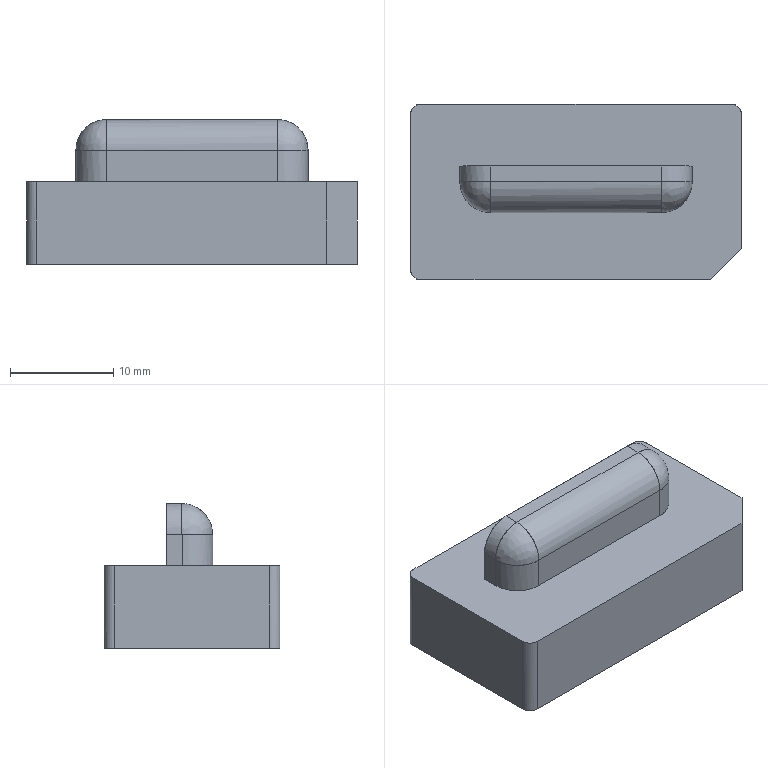NC program | PowerMill | posted with a generic post | part box 32 x 17 x 14 mm
Lines 6788 to 7532 of 64476:
N6885 M6
N6886 S22000 M03
N6887 G00 G90 X0.0 Y0.0
N6888 G43 Z10.8 H22
N6889
N6890 G05 P10000 R8
N6891 X11.5065 Y-1.9998
N6892 Z-3.6549
N6893 G01 Z-4.8549 F1200.0
N6894 X11.5064 Y-1.9999 Z-4.8359 F2000.0
N6895 X11.5061 Y-2.0002 Z-4.7481
N6896 X11.5052 Y-2.0011 Z-4.6724
N6897 X11.5043 Y-2.002 Z-4.6556
N6898 X11.5011 Y-2.0052 Z-4.637
N6899 X11.4961 Y-2.0102 Z-4.6202
N6900 X11.4874 Y-2.0189 Z-4.5995
N6901 X11.4751 Y-2.0312 Z-4.5776
N6902 X11.4577 Y-2.0486 Z-4.5522
N6903 X11.4357 Y-2.0706 Z-4.5218
N6904 X11.371 Y-2.1353 Z-4.4994
N6905 X11.3141 Y-2.1922 Z-4.513
N6906 X11.273 Y-2.2334 Z-4.5461
N6907 X11.2385 Y-2.2678 Z-4.6067
N6908 X11.2336 Y-2.2727 Z-4.6207
N6909 X11.2296 Y-2.2768 Z-4.6404
N6910 X11.2264 Y-2.2799 Z-4.6673
N6911 X11.2234 Y-2.2829 Z-4.6942
N6912 Z-4.8769
N6913 X11.1133 Y-2.3789 Z-4.8717
N6914 X11.0008 Y-2.4717 Z-4.8666
N6915 X10.8966 Y-2.5531 Z-4.862
N6916 X10.8967 Z-4.6977
N6917 X10.8987 Y-2.5511 Z-4.656
N6918 X10.9017 Y-2.548 Z-4.6144
N6919 X10.9065 Y-2.5432 Z-4.5719
N6920 X10.9133 Y-2.5364 Z-4.5313
N6921 X10.9222 Y-2.5275 Z-4.4917
N6922 X10.9329 Y-2.5169 Z-4.4528
N6923 X10.9446 Y-2.5052 Z-4.4156
N6924 X10.9582 Y-2.4915 Z-4.3799
N6925 X10.9752 Y-2.4746 Z-4.3427
N6926 X10.9959 Y-2.4539 Z-4.3043
N6927 X11.02 Y-2.4297 Z-4.2656
N6928 X11.0465 Y-2.4032 Z-4.2291
N6929 X11.0735 Y-2.3763 Z-4.1972
N6930 X11.0998 Y-2.3499 Z-4.1705
N6931 X11.1251 Y-2.3246 Z-4.1488
N6932 X11.1509 Y-2.2989 Z-4.1307
N6933 X11.184 Y-2.2657 Z-4.1113
N6934 X11.2182 Y-2.2315 Z-4.0957
N6935 X11.2532 Y-2.1965 Z-4.0839
N6936 X11.2888 Y-2.1609 Z-4.076
N6937 X11.3248 Y-2.1249 Z-4.0721
N6938 X11.3585 Y-2.0912
N6939 X11.3924 Y-2.0574 Z-4.0759
N6940 X11.4262 Y-2.0236 Z-4.0838
N6941 X11.4596 Y-1.9901 Z-4.0956
N6942 X11.4923 Y-1.9574 Z-4.1113
N6943 X11.5241 Y-1.9257 Z-4.1306
N6944 X11.5546 Y-1.8951 Z-4.1536
N6945 X11.5838 Y-1.866 Z-4.1798
N6946 X11.6111 Y-1.8387 Z-4.2088
N6947 X11.6365 Y-1.8132 Z-4.2391
N6948 X11.6603 Y-1.7894 Z-4.2716
N6949 X11.6822 Y-1.7676 Z-4.3066
N6950 X11.7013 Y-1.7484 Z-4.3431
N6951 X11.7181 Y-1.7317 Z-4.381
N6952 X11.7328 Y-1.717 Z-4.4203
N6953 X11.7453 Y-1.7045 Z-4.4594
N6954 X11.756 Y-1.6938 Z-4.5002
N6955 X11.7645 Y-1.6853 Z-4.542
N6956 X11.7708 Y-1.679 Z-4.5848
N6957 X11.7752 Y-1.6746 Z-4.6302
N6958 X11.7785 Y-1.6712 Z-4.6864
N6959 X11.7786 Y-1.6711 Z-4.6891
N6960 X11.7787 Y-1.671 Z-4.8532
N6961 X11.9152 Y-1.478 Z-4.8497
N6962 Z-4.691
N6963 X11.9149 Y-1.4783 Z-4.68
N6964 X11.9116 Y-1.4816 Z-4.6166
N6965 X11.9056 Y-1.4875 Z-4.5546
N6966 X11.8971 Y-1.4961 Z-4.4947
N6967 X11.887 Y-1.5062 Z-4.4412
N6968 X11.8739 Y-1.5193 Z-4.3876
N6969 X11.8581 Y-1.5351 Z-4.3347
N6970 X11.8402 Y-1.553 Z-4.2848
N6971 X11.8206 Y-1.5725 Z-4.2381
N6972 X11.7977 Y-1.5954 Z-4.1897
N6973 X11.7731 Y-1.6201 Z-4.1441
N6974 X11.7467 Y-1.6465 Z-4.1018
N6975 X11.7187 Y-1.6744 Z-4.0627
N6976 X11.6891 Y-1.704 Z-4.0267
N6977 X11.658 Y-1.7352 Z-3.9935
N6978 X11.6249 Y-1.7683 Z-3.9625
N6979 X11.5894 Y-1.8038 Z-3.9338
N6980 X11.5526 Y-1.8405 Z-3.9087
N6981 X11.5147 Y-1.8785 Z-3.8872
N6982 X11.4756 Y-1.9175 Z-3.8693
N6983 X11.4357 Y-1.9574 Z-3.8553
N6984 X11.3952 Y-1.998 Z-3.8451
N6985 X11.3541 Y-2.0391 Z-3.8389
N6986 X11.3128 Y-2.0804 Z-3.8366
N6987 X11.2715 Y-2.1217 Z-3.8383
N6988 X11.2304 Y-2.1628 Z-3.844
N6989 X11.19 Y-2.2032 Z-3.8536
N6990 X11.1501 Y-2.2431 Z-3.867
N6991 X11.1109 Y-2.2823 Z-3.8844
N6992 X11.0726 Y-2.3206 Z-3.9055
N6993 X11.0353 Y-2.3579 Z-3.9303
N6994 X10.9992 Y-2.3939 Z-3.9587
N6995 X10.9646 Y-2.4285 Z-3.9906
N6996 X10.9317 Y-2.4615 Z-4.0256
N6997 X10.9004 Y-2.4927 Z-4.0639
N6998 X10.8711 Y-2.5221 Z-4.1051
N6999 X10.8437 Y-2.5494 Z-4.149
N7000 X10.8185 Y-2.5747 Z-4.1957
N7001 X10.7955 Y-2.5977 Z-4.2447
N7002 X10.7749 Y-2.6183 Z-4.296
N7003 X10.7567 Y-2.6364 Z-4.3491
N7004 X10.7412 Y-2.652 Z-4.4038
N7005 X10.7283 Y-2.6649 Z-4.4599
N7006 X10.718 Y-2.6751 Z-4.5171
N7007 X10.7105 Y-2.6827 Z-4.5751
N7008 X10.7057 Y-2.6874 Z-4.6338
N7009 X10.7037 Y-2.6894 Z-4.6929
N7010 Y-2.6895 Z-4.8562
N7011 X10.5482 Y-2.7884 Z-4.8553
N7012 Z-4.6812
N7013 X10.5506 Y-2.786 Z-4.6155
N7014 X10.5558 Y-2.7808 Z-4.5504
N7015 X10.5638 Y-2.7728 Z-4.4862
N7016 X10.5745 Y-2.7621 Z-4.4231
N7017 X10.5879 Y-2.7487 Z-4.3612
N7018 X10.6038 Y-2.7328 Z-4.3009
N7019 X10.6224 Y-2.7142 Z-4.2422
N7020 X10.6434 Y-2.6932 Z-4.1854
N7021 X10.6668 Y-2.6698 Z-4.1307
N7022 X10.6925 Y-2.6441 Z-4.0781
N7023 X10.7205 Y-2.6161 Z-4.0278
N7024 X10.7508 Y-2.5858 Z-3.9797
N7025 X10.7828 Y-2.5538 Z-3.9346
N7026 X10.8165 Y-2.5201 Z-3.8924
N7027 X10.852 Y-2.4846 Z-3.8533
N7028 X10.889 Y-2.4476 Z-3.8174
N7029 X10.9275 Y-2.4091 Z-3.7849
N7030 X10.9674 Y-2.3692 Z-3.7557
N7031 X11.0087 Y-2.3279 Z-3.73
N7032 X11.0511 Y-2.2855 Z-3.7079
N7033 X11.0946 Y-2.242 Z-3.6895
N7034 X11.1391 Y-2.1975 Z-3.6748
N7035 X11.1843 Y-2.1523 Z-3.664
N7036 X11.2286 Y-2.1079 Z-3.6573
N7037 X11.2732 Y-2.0634 Z-3.6545
N7038 X11.3178 Y-2.0188 Z-3.6556
N7039 X11.3624 Y-1.9742 Z-3.6607
N7040 X11.4069 Y-1.9297 Z-3.6697
N7041 X11.4509 Y-1.8857 Z-3.6826
N7042 X11.4945 Y-1.8421 Z-3.6994
N7043 X11.5374 Y-1.7992 Z-3.7201
N7044 X11.5795 Y-1.7571 Z-3.7445
N7045 X11.6204 Y-1.7162 Z-3.7727
N7046 X11.6601 Y-1.6765 Z-3.8043
N7047 X11.6983 Y-1.6383 Z-3.8394
N7048 X11.7348 Y-1.6018 Z-3.8777
N7049 X11.7694 Y-1.5672 Z-3.9189
N7050 X11.8002 Y-1.5364 Z-3.9605
N7051 X11.8303 Y-1.5063 Z-4.0064
N7052 X11.8593 Y-1.4773 Z-4.0564
N7053 X11.8861 Y-1.4505 Z-4.1086
N7054 X11.9097 Y-1.4269 Z-4.1613
N7055 X11.9302 Y-1.4064 Z-4.214
N7056 X11.9486 Y-1.388 Z-4.2682
N7057 X11.9657 Y-1.3709 Z-4.3263
N7058 X11.9804 Y-1.3562 Z-4.3856
N7059 X11.9925 Y-1.3441 Z-4.446
N7060 X12.0018 Y-1.3348 Z-4.5075
N7061 X12.0085 Y-1.3281 Z-4.5697
N7062 X12.0126 Y-1.324 Z-4.6326
N7063 X12.0144 Y-1.3222 Z-4.6904
N7064 X12.0145 Y-1.3221 Z-4.8542
N7065 X12.0937 Y-1.1864 Z-4.8586
N7066 X12.0936 Z-4.6881
N7067 X12.0926 Y-1.1874 Z-4.642
N7068 X12.0895 Y-1.1906 Z-4.5798
N7069 X12.084 Y-1.196 Z-4.5179
N7070 X12.0757 Y-1.2043 Z-4.4546
N7071 X12.0653 Y-1.2147 Z-4.394
N7072 X12.0529 Y-1.2271 Z-4.3341
N7073 X12.0387 Y-1.2413 Z-4.275
N7074 X12.0206 Y-1.2594 Z-4.2111
N7075 X12.0001 Y-1.28 Z-4.1492
N7076 X11.9771 Y-1.3029 Z-4.0894
N7077 X11.9517 Y-1.3283 Z-4.0316
N7078 X11.9238 Y-1.3562 Z-3.9756
N7079 X11.8934 Y-1.3866 Z-3.9216
N7080 X11.8622 Y-1.4179 Z-3.872
N7081 X11.8289 Y-1.4511 Z-3.8248
N7082 X11.7932 Y-1.4869 Z-3.7798
N7083 X11.755 Y-1.5251 Z-3.737
N7084 X11.7153 Y-1.5647 Z-3.6975
N7085 X11.6743 Y-1.6058 Z-3.6614
N7086 X11.6318 Y-1.6482 Z-3.6287
N7087 X11.5881 Y-1.6919 Z-3.5995
N7088 X11.5432 Y-1.7368 Z-3.574
N7089 X11.4973 Y-1.7827 Z-3.5521
N7090 X11.4506 Y-1.8294 Z-3.5341
N7091 X11.4032 Y-1.8769 Z-3.5199
N7092 X11.3552 Y-1.9248 Z-3.5097
N7093 X11.3069 Y-1.9731 Z-3.5034
N7094 X11.2584 Y-2.0216 Z-3.5011
N7095 X11.2099 Y-2.0701 Z-3.5028
N7096 X11.1616 Y-2.1184 Z-3.5085
N7097 X11.1137 Y-2.1664 Z-3.5181
N7098 X11.0662 Y-2.2138 Z-3.5316
N7099 X11.0193 Y-2.2607 Z-3.549
N7100 X10.9733 Y-2.3067 Z-3.5701
N7101 X10.9281 Y-2.3519 Z-3.5951
N7102 X10.884 Y-2.3961 Z-3.6238
N7103 X10.8409 Y-2.4391 Z-3.6561
N7104 X10.7992 Y-2.4808 Z-3.692
N7105 X10.7589 Y-2.5212 Z-3.7314
N7106 X10.7201 Y-2.5599 Z-3.774
N7107 X10.6836 Y-2.5964 Z-3.8192
N7108 X10.6489 Y-2.6312 Z-3.8674
N7109 X10.6162 Y-2.6638 Z-3.9183
N7110 X10.5857 Y-2.6944 Z-3.9718
N7111 X10.5574 Y-2.7227 Z-4.0277
N7112 X10.5313 Y-2.7487 Z-4.086
N7113 X10.5076 Y-2.7724 Z-4.1464
N7114 X10.4864 Y-2.7936 Z-4.2088
N7115 X10.4677 Y-2.8123 Z-4.2729
N7116 X10.4517 Y-2.8284 Z-4.3385
N7117 X10.4383 Y-2.8417 Z-4.4054
N7118 X10.4276 Y-2.8524 Z-4.4732
N7119 X10.4198 Y-2.8603 Z-4.5418
N7120 X10.4147 Y-2.8653 Z-4.6109
N7121 X10.4124 Y-2.8676 Z-4.6803
N7122 Y-2.8677 Z-4.851
N7123 X10.2897 Y-2.9337 Z-4.8504
N7124 X10.2898 Z-4.6803
N7125 X10.2921 Y-2.9313 Z-4.6058
N7126 X10.2973 Y-2.9262 Z-4.5321
N7127 X10.3051 Y-2.9183 Z-4.4594
N7128 X10.3157 Y-2.9078 Z-4.3879
N7129 X10.3289 Y-2.8946 Z-4.3179
N7130 X10.3447 Y-2.8787 Z-4.2494
N7131 X10.3631 Y-2.8604 Z-4.1827
N7132 X10.384 Y-2.8395 Z-4.1176
N7133 X10.4081 Y-2.8154 Z-4.0521
N7134 X10.4346 Y-2.7889 Z-3.9886
N7135 X10.4634 Y-2.7601 Z-3.9275
N7136 X10.4944 Y-2.729 Z-3.8688
N7137 X10.5276 Y-2.6959 Z-3.8128
N7138 X10.5628 Y-2.6607 Z-3.7596
N7139 X10.5998 Y-2.6237 Z-3.7093
N7140 X10.6387 Y-2.5847 Z-3.6621
N7141 X10.6794 Y-2.544 Z-3.6179
N7142 X10.7218 Y-2.5016 Z-3.5769
N7143 X10.7657 Y-2.4577 Z-3.5393
N7144 X10.8111 Y-2.4124 Z-3.5052
N7145 X10.8578 Y-2.3657 Z-3.4745
N7146 X10.9056 Y-2.3179 Z-3.4475
N7147 X10.9544 Y-2.269 Z-3.4243
N7148 X11.0041 Y-2.2194 Z-3.4048
N7149 X11.0544 Y-2.1691 Z-3.3893
N7150 X11.1052 Y-2.1183 Z-3.3776
N7151 X11.1538 Y-2.0696 Z-3.3702
N7152 X11.2029 Y-2.0205 Z-3.3666
N7153 X11.2532 Y-1.9703 Z-3.3669
N7154 X11.3046 Y-1.9188 Z-3.3711
N7155 X11.3551 Y-1.8684 Z-3.379
N7156 X11.4052 Y-1.8182 Z-3.3908
N7157 X11.4549 Y-1.7686 Z-3.4065
N7158 X11.5038 Y-1.7196 Z-3.4261
N7159 X11.552 Y-1.6714 Z-3.4495
N7160 X11.5993 Y-1.6241 Z-3.4767
N7161 X11.6456 Y-1.5779 Z-3.5076
N7162 X11.6906 Y-1.5328 Z-3.5422
N7163 X11.7343 Y-1.4892 Z-3.5802
N7164 X11.7764 Y-1.4471 Z-3.6215
N7165 X11.8169 Y-1.4066 Z-3.6661
N7166 X11.8555 Y-1.3679 Z-3.7137
N7167 X11.8923 Y-1.3311 Z-3.7644
N7168 X11.9272 Y-1.2963 Z-3.8178
N7169 X11.9598 Y-1.2637 Z-3.8738
N7170 X11.9901 Y-1.2333 Z-3.9321
N7171 X12.0181 Y-1.2053 Z-3.9927
N7172 X12.044 Y-1.1795 Z-4.0558
N7173 X12.0674 Y-1.156 Z-4.1211
N7174 X12.0885 Y-1.135 Z-4.1884
N7175 X12.107 Y-1.1165 Z-4.2575
N7176 X12.1229 Y-1.1006 Z-4.3283
N7177 X12.1351 Y-1.0884 Z-4.3945
N7178 X12.1448 Y-1.0786 Z-4.4629
N7179 X12.1522 Y-1.0712 Z-4.5345
N7180 X12.1572 Y-1.0663 Z-4.6096
N7181 X12.1593 Y-1.0642 Z-4.6712
N7182 Y-1.0641 Z-4.8602
N7183 X12.2164 Y-0.9505 Z-4.8613
N7184 Z-4.6895
N7185 X12.2155 Y-0.9514 Z-4.6452
N7186 X12.2118 Y-0.9551 Z-4.5669
N7187 X12.2053 Y-0.9616 Z-4.4894
N7188 X12.1961 Y-0.9708 Z-4.413
N7189 X12.1842 Y-0.9827 Z-4.3378
N7190 X12.1697 Y-0.9972 Z-4.264
N7191 X12.1525 Y-1.0144 Z-4.1918
N7192 X12.1328 Y-1.0341 Z-4.1213
N7193 X12.1106 Y-1.0563 Z-4.0525
N7194 X12.0858 Y-1.0811 Z-3.9853
N7195 X12.0585 Y-1.1084 Z-3.92
N7196 X12.0288 Y-1.1381 Z-3.8567
N7197 X11.9966 Y-1.1703 Z-3.7956
N7198 X11.9622 Y-1.2047 Z-3.7367
N7199 X11.9255 Y-1.2414 Z-3.6801
N7200 X11.8877 Y-1.2791 Z-3.6278
N7201 X11.8481 Y-1.3188 Z-3.5783
N7202 X11.8066 Y-1.3603 Z-3.5318
N7203 X11.7632 Y-1.4037 Z-3.4883
N7204 X11.7181 Y-1.4488 Z-3.4479
N7205 X11.6715 Y-1.4954 Z-3.4109
N7206 X11.6234 Y-1.5434 Z-3.3774
N7207 X11.5741 Y-1.5928 Z-3.3474
N7208 X11.5238 Y-1.6431 Z-3.3211
N7209 X11.4726 Y-1.6943 Z-3.2986
N7210 X11.4207 Y-1.7462 Z-3.2801
N7211 X11.3682 Y-1.7987 Z-3.2654
N7212 X11.3155 Y-1.8514 Z-3.2547
N7213 X11.2625 Y-1.9044 Z-3.2479
N7214 X11.2096 Y-1.9573 Z-3.2451
N7215 X11.1567 Y-2.0102 Z-3.2463
N7216 X11.1041 Y-2.0628 Z-3.2515
N7217 X11.0504 Y-2.1165 Z-3.2606
N7218 X10.9974 Y-2.1695 Z-3.2737
N7219 X10.9453 Y-2.2216 Z-3.2906
N7220 X10.8941 Y-2.2728 Z-3.3113
N7221 X10.8438 Y-2.3231 Z-3.3357
N7222 X10.7944 Y-2.3725 Z-3.3639
N7223 X10.7461 Y-2.4208 Z-3.3959
N7224 X10.6988 Y-2.4681 Z-3.4315
N7225 X10.6545 Y-2.5124 Z-3.4692
N7226 X10.6102 Y-2.5567 Z-3.5114
N7227 X10.5665 Y-2.6004 Z-3.5577
N7228 X10.5248 Y-2.6421 Z-3.6069
N7229 X10.486 Y-2.6809 Z-3.6576
N7230 X10.4502 Y-2.7167 Z-3.7096
N7231 X10.4166 Y-2.7503 Z-3.7638
N7232 X10.3834 Y-2.7835 Z-3.8233
N7233 X10.352 Y-2.8149 Z-3.8859
N7234 X10.3228 Y-2.8441 Z-3.9511
N7235 X10.296 Y-2.8709 Z-4.0184
N7236 X10.2718 Y-2.895 Z-4.0871
N7237 X10.2505 Y-2.9164 Z-4.1567
N7238 X10.232 Y-2.9349 Z-4.2268
N7239 X10.2165 Y-2.9504 Z-4.2967
N7240 X10.205 Y-2.9619 Z-4.3595
N7241 X10.1953 Y-2.9716 Z-4.4229
N7242 X10.1874 Y-2.9794 Z-4.4868
N7243 X10.1819 Y-2.985 Z-4.5512
N7244 X10.1784 Y-2.9885 Z-4.6159
N7245 X10.1765 Y-2.9904 Z-4.6807
N7246 X10.1764 Z-4.8487
N7247 X10.0707 Y-3.0396 Z-4.8465
N7248 Z-4.6866
N7249 X10.0723 Y-3.0381 Z-4.6113
N7250 X10.0766 Y-3.0337 Z-4.5349
N7251 X10.0838 Y-3.0265 Z-4.4575
N7252 X10.0939 Y-3.0164 Z-4.3798
N7253 X10.1068 Y-3.0035 Z-4.3022
N7254 X10.1226 Y-2.9878 Z-4.2253
N7255 X10.1409 Y-2.9694 Z-4.1499
N7256 X10.1617 Y-2.9486 Z-4.0764
N7257 X10.1849 Y-2.9255 Z-4.0053
N7258 X10.2101 Y-2.9002 Z-3.9371
N7259 X10.2376 Y-2.8727 Z-3.8712
N7260 X10.2685 Y-2.8418 Z-3.8047
N7261 X10.3018 Y-2.8086 Z-3.7405
N7262 X10.3372 Y-2.7731 Z-3.6789
N7263 X10.3747 Y-2.7357 Z-3.62
N7264 X10.4141 Y-2.6962 Z-3.564
N7265 X10.4554 Y-2.6549 Z-3.511
N7266 X10.4984 Y-2.6119 Z-3.4611
N7267 X10.5431 Y-2.5672 Z-3.4145
N7268 X10.5892 Y-2.5211 Z-3.3713
N7269 X10.6369 Y-2.4735 Z-3.3314
N7270 X10.6858 Y-2.4245 Z-3.2951
N7271 X10.7366 Y-2.3737 Z-3.2618
N7272 X10.7884 Y-2.3219 Z-3.2323
N7273 X10.841 Y-2.2693 Z-3.2066
N7274 X10.8943 Y-2.216 Z-3.1848
N7275 X10.948 Y-2.1623 Z-3.1669
N7276 X11.0021 Y-2.1082 Z-3.153
N7277 X11.0564 Y-2.054 Z-3.1431
N7278 X11.1108 Y-1.9995 Z-3.1371
N7279 X11.1671 Y-1.9432 Z-3.1348
N7280 X11.223 Y-1.8873 Z-3.1364
N7281 X11.2783 Y-1.8321 Z-3.1419
N7282 X11.333 Y-1.7773 Z-3.1514
N7283 X11.3871 Y-1.7232 Z-3.1648
N7284 X11.4405 Y-1.6698 Z-3.1821
N7285 X11.4933 Y-1.6171 Z-3.2032
N7286 X11.5453 Y-1.5651 Z-3.2282
N7287 X11.5965 Y-1.5138 Z-3.257
N7288 X11.6469 Y-1.4634 Z-3.2896
N7289 X11.6965 Y-1.4138 Z-3.326
N7290 X11.7441 Y-1.3662 Z-3.3652
N7291 X11.7899 Y-1.3204 Z-3.4073
N7292 X11.8339 Y-1.2764 Z-3.4523
N7293 X11.8761 Y-1.2342 Z-3.5004
N7294 X11.9166 Y-1.1937 Z-3.5515
N7295 X11.9554 Y-1.1549 Z-3.6059
N7296 X11.9926 Y-1.1178 Z-3.6636
N7297 X12.0281 Y-1.0822 Z-3.7246
N7298 X12.0622 Y-1.0482 Z-3.7891
N7299 X12.0918 Y-1.0185 Z-3.8512
N7300 X12.1195 Y-0.9908 Z-3.9163
N7301 X12.1454 Y-0.9649 Z-3.9849
N7302 X12.1694 Y-0.9409 Z-4.0567
N7303 X12.1914 Y-0.9189 Z-4.1319
N7304 X12.208 Y-0.9023 Z-4.1966
N7305 X12.2223 Y-0.888 Z-4.2623
N7306 X12.2353 Y-0.875 Z-4.3338
N7307 X12.2469 Y-0.8635 Z-4.412
N7308 X12.2558 Y-0.8545 Z-4.4912
N7309 X12.2617 Y-0.8487 Z-4.5651
N7310 X12.2648 Y-0.8455 Z-4.6337
N7311 X12.2655 Y-0.8448 Z-4.6832
N7312 Z-4.8593
N7313 X12.3092 Y-0.7445 Z-4.8621
N7314 Y-0.7446 Z-4.6874
N7315 X12.3079 Y-0.7459 Z-4.6179
N7316 X12.3038 Y-0.7499 Z-4.5385
N7317 X12.2969 Y-0.7569 Z-4.4577
N7318 X12.287 Y-0.7667 Z-4.3762
N7319 X12.2743 Y-0.7794 Z-4.2947
N7320 X12.259 Y-0.7948 Z-4.2146
N7321 X12.2412 Y-0.8126 Z-4.1369
N7322 X12.2212 Y-0.8325 Z-4.0621
N7323 X12.1997 Y-0.8541 Z-3.9918
N7324 X12.1754 Y-0.8784 Z-3.9219
N7325 X12.1477 Y-0.9061 Z-3.8509
N7326 X12.1169 Y-0.9369 Z-3.7802
N7327 X12.0841 Y-0.9696 Z-3.7124
N7328 X12.0502 Y-1.0035 Z-3.649
N7329 X12.0158 Y-1.038 Z-3.5907
N7330 X11.9798 Y-1.074 Z-3.5357
N7331 X11.9387 Y-1.115 Z-3.4784
N7332 X11.8962 Y-1.1576 Z-3.4244
N7333 X11.8522 Y-1.2016 Z-3.374
N7334 X11.8067 Y-1.247 Z-3.3269
N7335 X11.7598 Y-1.294 Z-3.2832
N7336 X11.7112 Y-1.3425 Z-3.2425
N7337 X11.6604 Y-1.3934 Z-3.2043
N7338 X11.6086 Y-1.4451 Z-3.1699
N7339 X11.556 Y-1.4977 Z-3.1393
N7340 X11.5026 Y-1.5512 Z-3.1126
N7341 X11.4483 Y-1.6055 Z-3.0896
N7342 X11.3932 Y-1.6606 Z-3.0705
N7343 X11.3373 Y-1.7164 Z-3.0552
N7344 X11.2807 Y-1.7731 Z-3.0437
N7345 X11.2233 Y-1.8305 Z-3.0362
N7346 X11.1652 Y-1.8886 Z-3.0325
N7347 X11.1063 Y-1.9474 Z-3.0327
N7348 X11.0568 Y-1.9969 Z-3.0361
N7349 X11.0075 Y-2.0463 Z-3.043
N7350 X10.9536 Y-2.1001 Z-3.054
N7351 X10.8963 Y-2.1575 Z-3.0696
N7352 X10.8445 Y-2.2092 Z-3.0871
N7353 X10.7969 Y-2.2569 Z-3.1064
N7354 X10.7499 Y-2.3039 Z-3.1288
N7355 X10.6955 Y-2.3583 Z-3.1588
N7356 X10.6424 Y-2.4114 Z-3.1923
N7357 X10.5907 Y-2.463 Z-3.2293
N7358 X10.5406 Y-2.5131 Z-3.2696
N7359 X10.4922 Y-2.5616 Z-3.3132
N7360 X10.4454 Y-2.6083 Z-3.3599
N7361 X10.4008 Y-2.6529 Z-3.4093
N7362 X10.3576 Y-2.6961 Z-3.4622
N7363 X10.3158 Y-2.7379 Z-3.5187
N7364 X10.2755 Y-2.7783 Z-3.5787
N7365 X10.239 Y-2.8148 Z-3.6384
N7366 X10.2043 Y-2.8494 Z-3.701
N7367 X10.1714 Y-2.8824 Z-3.767
N7368 X10.1403 Y-2.9135 Z-3.8363
N7369 X10.1116 Y-2.9422 Z-3.9074
N7370 X10.0855 Y-2.9683 Z-3.9802
N7371 X10.0619 Y-2.9918 Z-4.0545
N7372 X10.041 Y-3.0127 Z-4.1303
N7373 X10.0228 Y-3.031 Z-4.2074
N7374 X10.0072 Y-3.0465 Z-4.2858
N7375 X9.9944 Y-3.0594 Z-4.3654
N7376 X9.9842 Y-3.0695 Z-4.4461
N7377 X9.9768 Y-3.077 Z-4.5278
N7378 X9.9722 Y-3.0816 Z-4.6104
N7379 X9.9703 Y-3.0835 Z-4.6937
N7380 X9.9702 Z-4.8448
N7381 X9.8749 Y-3.1223 Z-4.8454
N7382 X9.875 Y-3.1222 Z-4.6989
N7383 X9.8766 Y-3.1206 Z-4.6133
N7384 X9.881 Y-3.1162 Z-4.5287
N7385 X9.8882 Y-3.109 Z-4.4453
N7386 X9.898 Y-3.0992 Z-4.3633
N7387 X9.9105 Y-3.0867 Z-4.2827
N7388 X9.9256 Y-3.0716 Z-4.2035
N7389 X9.9437 Y-3.0535 Z-4.1227
N7390 X9.964 Y-3.0332 Z-4.0446
N7391 X9.9866 Y-3.0105 Z-3.969
N7392 X10.0116 Y-2.9856 Z-3.8959
N7393 X10.0388 Y-2.9584 Z-3.825
N7394 X10.0682 Y-2.929 Z-3.7562
N7395 X10.0982 Y-2.899 Z-3.6923
N7396 X10.1298 Y-2.8674 Z-3.6301
N7397 X10.1634 Y-2.8338 Z-3.57
N7398 X10.199 Y-2.7982 Z-3.5121
N7399 X10.2364 Y-2.7608 Z-3.4566
N7400 X10.2753 Y-2.7219 Z-3.4033
N7401 X10.3178 Y-2.6794 Z-3.3498
N7402 X10.3629 Y-2.6343 Z-3.2984
N7403 X10.4102 Y-2.587 Z-3.2496
N7404 X10.4597 Y-2.5375 Z-3.2036
N7405 X10.5109 Y-2.4863 Z-3.1606
N7406 X10.5635 Y-2.4337 Z-3.1211
N7407 X10.6172 Y-2.38 Z-3.0854
N7408 X10.6715 Y-2.3257 Z-3.0535
N7409 X10.7263 Y-2.2709 Z-3.0257
N7410 X10.7828 Y-2.2144 Z-3.0011
N7411 X10.84 Y-2.1572 Z-2.9805
N7412 X10.8976 Y-2.0996 Z-2.9638
N7413 X10.9556 Y-2.0416 Z-2.9511
N7414 X11.0138 Y-1.9834 Z-2.9423
N7415 X11.0721 Y-1.9251 Z-2.9376
N7416 X11.1304 Y-1.8668 Z-2.9368
N7417 X11.1896 Y-1.8076 Z-2.9398
N7418 X11.2484 Y-1.7488 Z-2.9469
N7419 X11.3069 Y-1.6903 Z-2.9578
N7420 X11.3648 Y-1.6324 Z-2.9727
N7421 X11.4221 Y-1.5751 Z-2.9915
N7422 X11.4786 Y-1.5186 Z-3.0141
N7423 X11.5343 Y-1.4629 Z-3.0405
N7424 X11.5889 Y-1.4082 Z-3.0707
N7425 X11.6425 Y-1.3547 Z-3.1045
N7426 X11.6949 Y-1.3023 Z-3.142
N7427 X11.7459 Y-1.2513 Z-3.1829
N7428 X11.7956 Y-1.2016 Z-3.2274
N7429 X11.8437 Y-1.1535 Z-3.2752
N7430 X11.8903 Y-1.1069 Z-3.3262
N7431 X11.9341 Y-1.0631 Z-3.3791
N7432 X11.9771 Y-1.0201 Z-3.4361
N7433 X12.0179 Y-0.9793 Z-3.4958
N7434 X12.0565 Y-0.9407 Z-3.5578
N7435 X12.0927 Y-0.9045 Z-3.6219
N7436 X12.1262 Y-0.8709 Z-3.6878
N7437 X12.1568 Y-0.8403 Z-3.7544
N7438 X12.1819 Y-0.8153 Z-3.8133
N7439 X12.2056 Y-0.7916 Z-3.8733
N7440 X12.2274 Y-0.7698 Z-3.9347
N7441 X12.2471 Y-0.7501 Z-3.9975
N7442 X12.2651 Y-0.732 Z-4.0613
N7443 X12.2816 Y-0.7155 Z-4.1259
N7444 X12.2981 Y-0.6991 Z-4.2012
N7445 X12.3129 Y-0.6843 Z-4.2822
N7446 X12.3257 Y-0.6715 Z-4.3667
N7447 X12.3355 Y-0.6617 Z-4.4501
N7448 X12.3425 Y-0.6547 Z-4.5323
N7449 X12.3465 Y-0.6507 Z-4.6133
N7450 X12.3477 Y-0.6495 Z-4.6697
N7451 Z-4.8706
N7452 X12.3822 Y-0.5584 Z-4.8755
N7453 X12.3821 Y-0.5585 Z-4.6534
N7454 X12.3811 Y-0.5595 Z-4.6137
N7455 X12.3774 Y-0.5633 Z-4.533
N7456 X12.3712 Y-0.5695 Z-4.4525
N7457 X12.3624 Y-0.5782 Z-4.3725
N7458 X12.3512 Y-0.5894 Z-4.2932
N7459 X12.3377 Y-0.6029 Z-4.2145
N7460 X12.3208 Y-0.6198 Z-4.1318
N7461 X12.3012 Y-0.6394 Z-4.0502
N7462 X12.2789 Y-0.6617 Z-3.97
N7463 X12.254 Y-0.6866 Z-3.8914
N7464 X12.2266 Y-0.714 Z-3.8146
N7465 X12.1968 Y-0.7439 Z-3.7398
N7466 X12.1644 Y-0.7762 Z-3.6669
N7467 X12.1298 Y-0.8108 Z-3.5963
N7468 X12.0931 Y-0.8475 Z-3.5285
N7469 X12.0542 Y-0.8864 Z-3.4632
N7470 X12.0132 Y-0.9274 Z-3.4006
N7471 X11.9702 Y-0.9704 Z-3.3407
N7472 X11.9252 Y-1.0154 Z-3.2838
N7473 X11.8784 Y-1.0622 Z-3.2299
N7474 X11.8299 Y-1.1108 Z-3.1791
N7475 X11.7797 Y-1.161 Z-3.1316
N7476 X11.7279 Y-1.2127 Z-3.0875
N7477 X11.6748 Y-1.2658 Z-3.0468
N7478 X11.6205 Y-1.3202 Z-3.0097
N7479 X11.5649 Y-1.3757 Z-2.9762
N7480 X11.5084 Y-1.4323 Z-2.9465
N7481 X11.4509 Y-1.4897 Z-2.9205
N7482 X11.3926 Y-1.548 Z-2.8984
N7483 X11.3343 Y-1.6063 Z-2.8803
N7484 X11.2754 Y-1.6652 Z-2.8661
N7485 X11.2157 Y-1.7249 Z-2.8557
N7486 X11.1553 Y-1.7853 Z-2.8493
N7487 X11.0944 Y-1.8462 Z-2.8468
N7488 X11.0346 Y-1.906 Z-2.8482
N7489 X10.9748 Y-1.9658 Z-2.8537
N7490 X10.9149 Y-2.0257 Z-2.8631
N7491 X10.8551 Y-2.0855 Z-2.8765
N7492 X10.7956 Y-2.145 Z-2.8939
N7493 X10.7365 Y-2.2042 Z-2.9153
N7494 X10.6791 Y-2.2615 Z-2.9401
N7495 X10.6224 Y-2.3182 Z-2.9688
N7496 X10.5665 Y-2.3741 Z-3.0013
N7497 X10.5116 Y-2.429 Z-3.0375
N7498 X10.4578 Y-2.4828 Z-3.0774
N7499 X10.4054 Y-2.5352 Z-3.1209
N7500 X10.3545 Y-2.5861 Z-3.1676
N7501 X10.3054 Y-2.6352 Z-3.2175
N7502 X10.2581 Y-2.6825 Z-3.2705
N7503 X10.2122 Y-2.7284 Z-3.3269
N7504 X10.1682 Y-2.7724 Z-3.3863
N7505 X10.1262 Y-2.8144 Z-3.4485
N7506 X10.0863 Y-2.8544 Z-3.5134
N7507 X10.0485 Y-2.8921 Z-3.5809
N7508 X10.0131 Y-2.9275 Z-3.6507
N7509 X9.98 Y-2.9606 Z-3.7226
N7510 X9.9494 Y-2.9913 Z-3.7966
N7511 X9.9212 Y-3.0194 Z-3.8725
N7512 X9.8956 Y-3.045 Z-3.9501
N7513 X9.8732 Y-3.0674 Z-4.0269
N7514 X9.8533 Y-3.0873 Z-4.1041
N7515 X9.8357 Y-3.1049 Z-4.1826
N7516 X9.8205 Y-3.1201 Z-4.2625
N7517 X9.8079 Y-3.1327 Z-4.3439
N7518 X9.798 Y-3.1426 Z-4.4268
N7519 X9.7908 Y-3.1498 Z-4.5105
N7520 X9.7862 Y-3.1544 Z-4.5948
N7521 X9.784 Y-3.1567 Z-4.6795
N7522 X9.7839 Z-4.8459
N7523 X9.6961 Y-3.1879 Z-4.8559
N7524 X9.6962 Y-3.1878 Z-4.6808
N7525 X9.6984 Y-3.1856 Z-4.5913
N7526 X9.7034 Y-3.1806 Z-4.5027
N7527 X9.7111 Y-3.1729 Z-4.4151
N7528 X9.7216 Y-3.1625 Z-4.3285
N7529 X9.7347 Y-3.1493 Z-4.2428
N7530 X9.7507 Y-3.1333 Z-4.1579
N7531 X9.7694 Y-3.1146 Z-4.0738
N7532 X9.7909 Y-3.0931 Z-3.9906
N7533 X9.8152 Y-3.0688 Z-3.9081
N7534 X9.8401 Y-3.044 Z-3.8332
N7535 X9.8679 Y-3.0162 Z-3.7586
N7536 X9.8989 Y-2.9851 Z-3.6837
N7537 X9.933 Y-2.951 Z-3.6093
N7538 X9.9698 Y-2.9142 Z-3.5362
N7539 X10.0087 Y-2.8754 Z-3.4659
N7540 X10.0489 Y-2.8351 Z-3.3994
N7541 X10.0901 Y-2.794 Z-3.3372
N7542 X10.1319 Y-2.7521 Z-3.2794
N7543 X10.1756 Y-2.7084 Z-3.2244
N7544 X10.2229 Y-2.6612 Z-3.17
N7545 X10.2729 Y-2.6112 Z-3.1176
N7546 X10.3251 Y-2.5589 Z-3.0678
N7547 X10.379 Y-2.5051 Z-3.0212
N7548 X10.4337 Y-2.4504 Z-2.9786
N7549 X10.4887 Y-2.3954 Z-2.9401
N7550 X10.5435 Y-2.3406 Z-2.9061
N7551 X10.599 Y-2.285 Z-2.8758
N7552 X10.6577 Y-2.2264 Z-2.8479
N7553 X10.717 Y-2.1671 Z-2.824
N7554 X10.7769 Y-2.1072 Z-2.8039
N7555 X10.8374 Y-2.0466 Z-2.7878
N7556 X10.8986 Y-1.9854 Z-2.7755
N7557 X10.9604 Y-1.9236 Z-2.7671
N7558 X11.0223 Y-1.8618 Z-2.7627
N7559 X11.0841 Y-1.7999 Z-2.7622
N7560 X11.1457 Y-1.7383 Z-2.7657
N7561 X11.207 Y-1.677 Z-2.7732
N7562 X11.2679 Y-1.6162 Z-2.7846
N7563 X11.3283 Y-1.5558 Z-2.8
N7564 X11.3881 Y-1.4959 Z-2.8193
N7565 X11.4473 Y-1.4367 Z-2.8424
N7566 X11.5058 Y-1.3783 Z-2.8693
N7567 X11.5639 Y-1.3201 Z-2.9002
N7568 X11.6207 Y-1.2633 Z-2.9346
N7569 X11.6761 Y-1.2079 Z-2.9725
N7570 X11.7301 Y-1.154 Z-3.0139
N7571 X11.7826 Y-1.1014 Z-3.0587
N7572 X11.8337 Y-1.0504 Z-3.1069
N7573 X11.8832 Y-1.0009 Z-3.1584
N7574 X11.9312 Y-0.9529 Z-3.2133
N7575 X11.9776 Y-0.9065 Z-3.2715
N7576 X12.0211 Y-0.863 Z-3.3313
N7577 X12.0628 Y-0.8212 Z-3.3942
N7578 X12.1028 Y-0.7812 Z-3.4603
N7579 X12.141 Y-0.7431 Z-3.5294
N7580 X12.1772 Y-0.7069 Z-3.6015
N7581 X12.2113 Y-0.6727 Z-3.6764
N7582 X12.2416 Y-0.6424 Z-3.7498
N7583 X12.2697 Y-0.6143 Z-3.8259
N7584 X12.2957 Y-0.5883 Z-3.9048
N7585 X12.3196 Y-0.5645 Z-3.9865
N7586 X12.3409 Y-0.5432 Z-4.07
N7587 X12.3596 Y-0.5245 Z-4.1548
N7588 X12.3755 Y-0.5085 Z-4.2408
N7589 X12.3887 Y-0.4953 Z-4.3277
N7590 X12.3992 Y-0.4849 Z-4.4153
N7591 X12.4068 Y-0.4772 Z-4.5035
N7592 X12.4116 Y-0.4724 Z-4.592
N7593 X12.4136 Y-0.4704 Z-4.6806
N7594 Z-4.6815
N7595 X12.4137 Z-4.8778
N7596 X12.4417 Y-0.3858 Z-4.8798
N7597 X12.4416 Y-0.3859 Z-4.6655
N7598 X12.4406 Y-0.3869 Z-4.6115
N7599 X12.4367 Y-0.3907 Z-4.5274
N7600 X12.4299 Y-0.3976 Z-4.4378
N7601 X12.4216 Y-0.4058 Z-4.3574
N7602 X12.4107 Y-0.4167 Z-4.2754
N7603 X12.3969 Y-0.4306 Z-4.1913
N7604 X12.3796 Y-0.4478 Z-4.1038
N7605 X12.3599 Y-0.4676 Z-4.0178
N7606 X12.3388 Y-0.4887 Z-3.9376
N7607 X12.3158 Y-0.5117 Z-3.8607
N7608 X12.2887 Y-0.5388 Z-3.7799
N7609 X12.259 Y-0.5685 Z-3.7008
N7610 X12.2268 Y-0.6007 Z-3.6237
N7611 X12.1922 Y-0.6353 Z-3.5486
N7612 X12.1553 Y-0.6722 Z-3.4757
N7613 X12.116 Y-0.7115 Z-3.4052
N7614 X12.0746 Y-0.7529 Z-3.3372
N7615 X12.0316 Y-0.7959 Z-3.2726
N7616 X11.9866 Y-0.8409 Z-3.2109
N7617 X11.9397 Y-0.8878 Z-3.152
N7618 X11.891 Y-0.9365 Z-3.0963
N7619 X11.8405 Y-0.987 Z-3.0435
N7620 X11.7882 Y-1.0393 Z-2.994
N7621 X11.7343 Y-1.0932 Z-2.9477
N7622 X11.6788 Y-1.1487 Z-2.9047
N7623 X11.6226 Y-1.2049 Z-2.8657
N7624 X11.5652 Y-1.2623 Z-2.8302
N7625 X11.5066 Y-1.3209 Z-2.7984
N7626 X11.4469 Y-1.3806 Z-2.7702
N7627 X11.3862 Y-1.4412 Z-2.7458
N7628 X11.3248 Y-1.5027 Z-2.7252
N7629 X11.2628 Y-1.5647 Z-2.7085